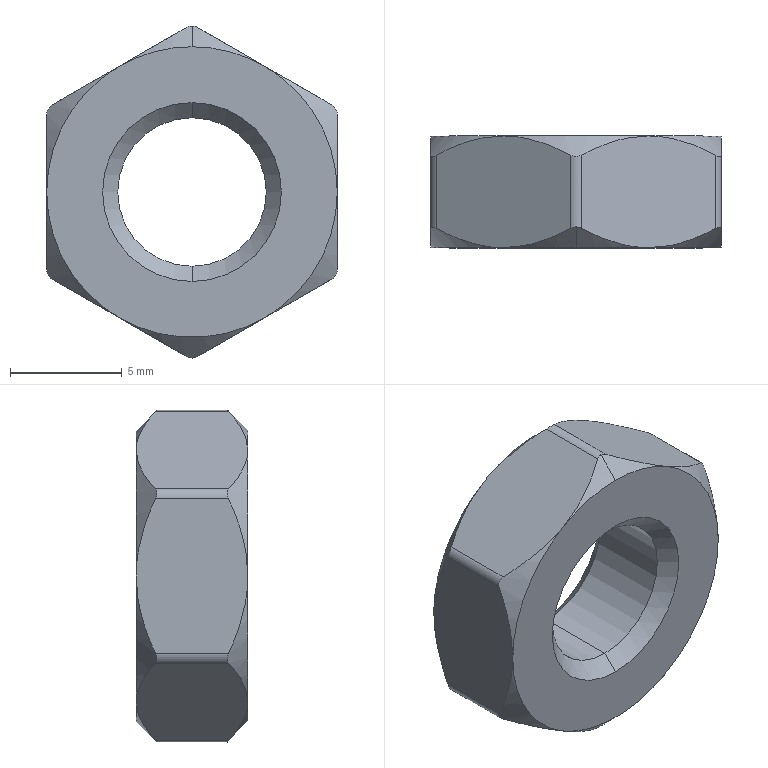Part | STEP file | TDB71-M8-L20-002^TDB71-M8-L20_Cylinder clamp assembly | 1 solid | 35 faces | box 13 x 5 x 14.854 mm | volume 539.687 mm3 | cone 18 | cylinder 9 | plane 8 | commonest cylinder face diameters 1 x7 6.647 x2